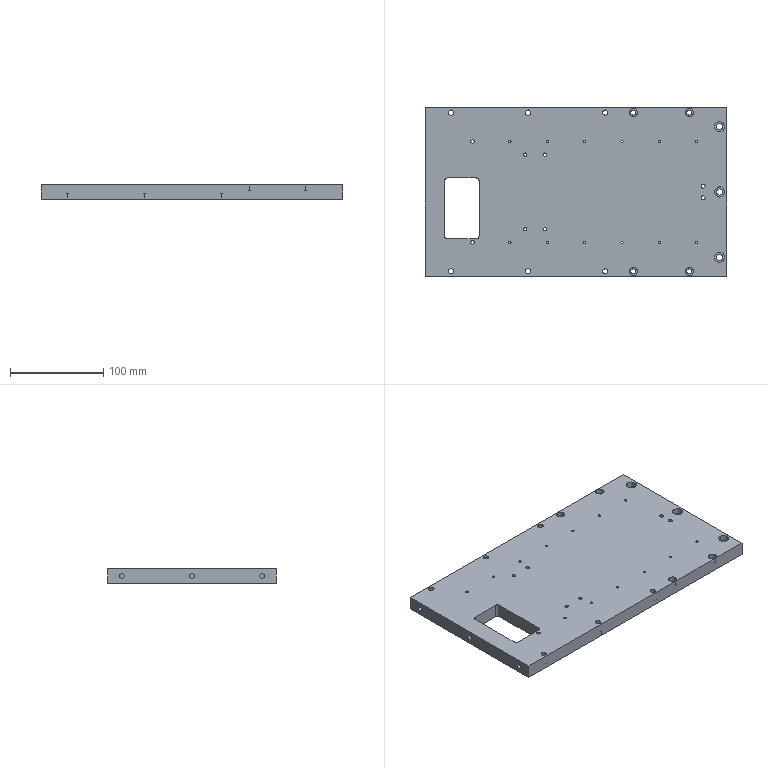Part | STEP file | PN_0003 | 1 solid | 127 faces | box 322.5 x 180 x 15 mm | volume 822668 mm3 | cylinder 102 | plane 25 | commonest cylinder face diameters 2.5 x24 5.5 x20 9 x20 3.5 x12 5 x6 6.5 x6